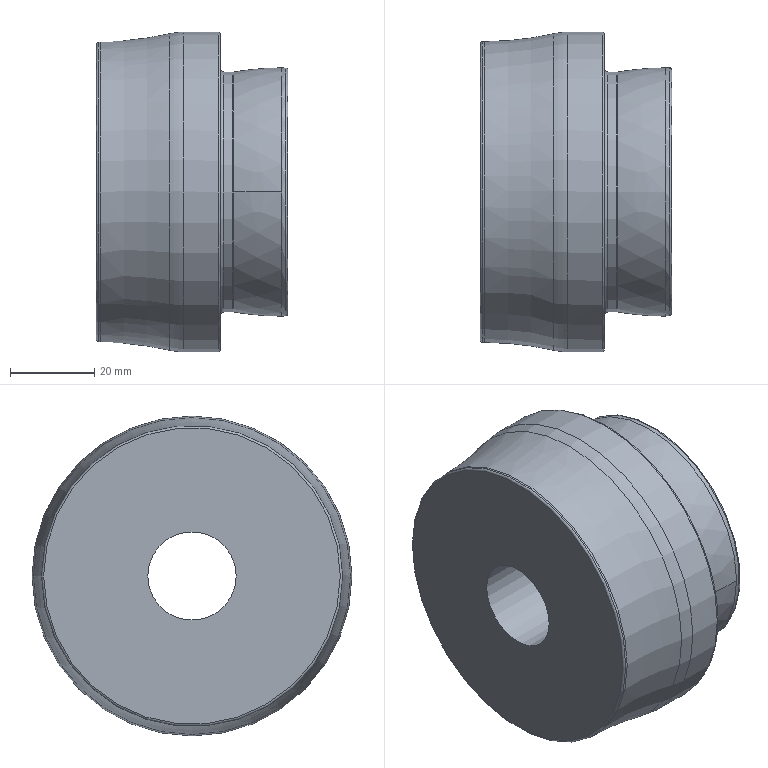Part | STEP file | P1317200001_D | 1 solid | 19 faces | box 45.5 x 76 x 76 mm | volume 152294 mm3 | torus 7 | cylinder 6 | plane 4 | spline 2 | commonest cylinder face diameters 21 x1 37 x1 57 x1 59 x1 71.5 x1 76 x1
STEP:
#1=CARTESIAN_POINT('',(0.,29.,0.));
#2=VERTEX_POINT('',#1);
#3=CARTESIAN_POINT('',(0.,28.999,-0.1765));
#4=VERTEX_POINT('',#3);
#5=CARTESIAN_POINT('',(0.,0.,0.));
#6=DIRECTION('',(1.,0.,0.));
#7=DIRECTION('',(0.,-1.,0.));
#8=AXIS2_PLACEMENT_3D('',#5,#6,#7);
#9=CIRCLE('',#8,29.);
#10=EDGE_CURVE('',#2,#4,#9,.T.);
#11=ORIENTED_EDGE('',*,*,#10,.T.);
#12=CARTESIAN_POINT('',(0.,0.,0.));
#13=DIRECTION('',(1.,0.,0.));
#14=DIRECTION('',(0.,-1.,0.));
#15=AXIS2_PLACEMENT_3D('',#12,#13,#14);
#16=CIRCLE('',#15,29.);
#17=EDGE_CURVE('',#4,#2,#16,.T.);
#18=ORIENTED_EDGE('',*,*,#17,.T.);
#19=EDGE_LOOP('',(#11,#18));
#20=FACE_OUTER_BOUND('',#19,.T.);
#21=CARTESIAN_POINT('',(0.,-18.5,0.));
#22=VERTEX_POINT('',#21);
#23=CARTESIAN_POINT('',(0.,0.,0.));
#24=DIRECTION('',(-1.,0.,0.));
#25=DIRECTION('',(0.,1.,0.));
#26=AXIS2_PLACEMENT_3D('',#23,#24,#25);
#27=CIRCLE('',#26,18.5);
#28=EDGE_CURVE('',#22,#22,#27,.T.);
#29=ORIENTED_EDGE('',*,*,#28,.T.);
#30=EDGE_LOOP('',(#29));
#31=FACE_BOUND('',#30,.T.);
#32=CARTESIAN_POINT('',(0.,0.,0.));
#33=DIRECTION('',(1.,0.,0.));
#34=DIRECTION('',(0.,-1.,0.));
#35=AXIS2_PLACEMENT_3D('',#32,#33,#34);
#36=PLANE('',#35);
#37=ADVANCED_FACE('',(#20,#31),#36,.T.);
#38=ORIENTED_EDGE('',*,*,#28,.F.);
#39=CARTESIAN_POINT('',(-2.,-18.5,0.));
#40=VERTEX_POINT('',#39);
#41=CARTESIAN_POINT('',(0.1,-18.5,0.));
#42=DIRECTION('',(-1.,0.,0.));
#43=VECTOR('',#42,18.5);
#44=LINE('',#41,#43);
#45=EDGE_CURVE('',#22,#40,#44,.T.);
#46=ORIENTED_EDGE('',*,*,#45,.T.);
#47=CARTESIAN_POINT('',(-2.,0.,0.));
#48=DIRECTION('',(-1.,0.,0.));
#49=DIRECTION('',(0.,1.,0.));
#50=AXIS2_PLACEMENT_3D('',#47,#48,#49);
#51=CIRCLE('',#50,18.5);
#52=EDGE_CURVE('',#40,#40,#51,.T.);
#53=ORIENTED_EDGE('',*,*,#52,.T.);
#54=ORIENTED_EDGE('',*,*,#45,.F.);
#55=EDGE_LOOP('',(#38,#46,#53,#54));
#56=FACE_OUTER_BOUND('',#55,.T.);
#57=CARTESIAN_POINT('',(0.1,0.,0.));
#58=DIRECTION('',(-1.,0.,0.));
#59=DIRECTION('',(0.,1.,0.));
#60=AXIS2_PLACEMENT_3D('',#57,#58,#59);
#61=CYLINDRICAL_SURFACE('',#60,18.5);
#62=ADVANCED_FACE('',(#56),#61,.F.);
#63=ORIENTED_EDGE('',*,*,#52,.F.);
#64=EDGE_LOOP('',(#63));
#65=FACE_OUTER_BOUND('',#64,.T.);
#66=CARTESIAN_POINT('',(-2.,-10.5,0.));
#67=VERTEX_POINT('',#66);
#68=CARTESIAN_POINT('',(-2.,10.5,0.));
#69=VERTEX_POINT('',#68);
#70=CARTESIAN_POINT('',(-2.,0.,0.));
#71=DIRECTION('',(-1.,0.,0.));
#72=DIRECTION('',(0.,1.,0.));
#73=AXIS2_PLACEMENT_3D('',#70,#71,#72);
#74=CIRCLE('',#73,10.5);
#75=EDGE_CURVE('',#67,#69,#74,.T.);
#76=ORIENTED_EDGE('',*,*,#75,.T.);
#77=CARTESIAN_POINT('',(-2.,0.,0.));
#78=DIRECTION('',(-1.,0.,0.));
#79=DIRECTION('',(0.,1.,0.));
#80=AXIS2_PLACEMENT_3D('',#77,#78,#79);
#81=CIRCLE('',#80,10.5);
#82=EDGE_CURVE('',#69,#67,#81,.T.);
#83=ORIENTED_EDGE('',*,*,#82,.T.);
#84=EDGE_LOOP('',(#76,#83));
#85=FACE_BOUND('',#84,.T.);
#86=CARTESIAN_POINT('',(-2.,0.,0.));
#87=DIRECTION('',(-1.,0.,0.));
#88=DIRECTION('',(0.,1.,0.));
#89=AXIS2_PLACEMENT_3D('',#86,#87,#88);
#90=PLANE('',#89);
#91=ADVANCED_FACE('',(#65,#85),#90,.F.);
#92=CARTESIAN_POINT('',(-45.5,-10.5,0.));
#93=VERTEX_POINT('',#92);
#94=CARTESIAN_POINT('',(-45.5,10.5,0.));
#95=VERTEX_POINT('',#94);
#96=CARTESIAN_POINT('',(-45.5,0.,0.));
#97=DIRECTION('',(-1.,0.,0.));
#98=DIRECTION('',(0.,1.,0.));
#99=AXIS2_PLACEMENT_3D('',#96,#97,#98);
#100=CIRCLE('',#99,10.5);
#101=EDGE_CURVE('',#93,#95,#100,.T.);
#102=ORIENTED_EDGE('',*,*,#101,.T.);
#103=CARTESIAN_POINT('',(-47.775,10.5,0.));
#104=DIRECTION('',(1.,0.,0.));
#105=VECTOR('',#104,10.5);
#106=LINE('',#103,#105);
#107=EDGE_CURVE('',#95,#69,#106,.T.);
#108=ORIENTED_EDGE('',*,*,#107,.T.);
#109=ORIENTED_EDGE('',*,*,#75,.F.);
#110=ORIENTED_EDGE('',*,*,#82,.F.);
#111=ORIENTED_EDGE('',*,*,#107,.F.);
#112=CARTESIAN_POINT('',(-45.5,0.,0.));
#113=DIRECTION('',(-1.,0.,0.));
#114=DIRECTION('',(0.,1.,0.));
#115=AXIS2_PLACEMENT_3D('',#112,#113,#114);
#116=CIRCLE('',#115,10.5);
#117=EDGE_CURVE('',#95,#93,#116,.T.);
#118=ORIENTED_EDGE('',*,*,#117,.T.);
#119=EDGE_LOOP('',(#102,#108,#109,#110,#111,#118));
#120=FACE_OUTER_BOUND('',#119,.T.);
#121=CARTESIAN_POINT('',(-47.775,0.,0.));
#122=DIRECTION('',(1.,0.,0.));
#123=DIRECTION('',(0.,-1.,0.));
#124=AXIS2_PLACEMENT_3D('',#121,#122,#123);
#125=CYLINDRICAL_SURFACE('',#124,10.5);
#126=ADVANCED_FACE('',(#120),#125,.F.);
#127=CARTESIAN_POINT('',(-45.5,35.25,0.));
#128=VERTEX_POINT('',#127);
#129=CARTESIAN_POINT('',(-45.5,35.249,0.2514));
#130=VERTEX_POINT('',#129);
#131=CARTESIAN_POINT('',(-45.5,0.,0.));
#132=DIRECTION('',(-1.,0.,0.));
#133=DIRECTION('',(0.,-1.,0.));
#134=AXIS2_PLACEMENT_3D('',#131,#132,#133);
#135=CIRCLE('',#134,35.25);
#136=EDGE_CURVE('',#128,#130,#135,.T.);
#137=ORIENTED_EDGE('',*,*,#136,.T.);
#138=CARTESIAN_POINT('',(-45.5,0.,0.));
#139=DIRECTION('',(-1.,0.,0.));
#140=DIRECTION('',(0.,-1.,0.));
#141=AXIS2_PLACEMENT_3D('',#138,#139,#140);
#142=CIRCLE('',#141,35.25);
#143=EDGE_CURVE('',#130,#128,#142,.T.);
#144=ORIENTED_EDGE('',*,*,#143,.T.);
#145=EDGE_LOOP('',(#137,#144));
#146=FACE_OUTER_BOUND('',#145,.T.);
#147=ORIENTED_EDGE('',*,*,#101,.F.);
#148=ORIENTED_EDGE('',*,*,#117,.F.);
#149=EDGE_LOOP('',(#147,#148));
#150=FACE_BOUND('',#149,.T.);
#151=CARTESIAN_POINT('',(-45.5,0.,0.));
#152=DIRECTION('',(1.,0.,0.));
#153=DIRECTION('',(0.,-1.,0.));
#154=AXIS2_PLACEMENT_3D('',#151,#152,#153);
#155=PLANE('',#154);
#156=ADVANCED_FACE('',(#146,#150),#155,.F.);
#157=CARTESIAN_POINT('',(-45.,35.75,0.));
#158=VERTEX_POINT('',#157);
#159=CARTESIAN_POINT('',(-45.,35.749,0.255));
#160=VERTEX_POINT('',#159);
#161=CARTESIAN_POINT('',(-45.,0.,0.));
#162=DIRECTION('',(-1.,0.,0.));
#163=DIRECTION('',(0.,-1.,0.));
#164=AXIS2_PLACEMENT_3D('',#161,#162,#163);
#165=CIRCLE('',#164,35.75);
#166=EDGE_CURVE('',#158,#160,#165,.T.);
#167=ORIENTED_EDGE('',*,*,#166,.T.);
#168=CARTESIAN_POINT('',(-45.,35.249,0.2514));
#169=DIRECTION('',(0.,-0.007133,1.));
#170=DIRECTION('',(0.,1.,0.007133));
#171=AXIS2_PLACEMENT_3D('',#168,#169,#170);
#172=CIRCLE('',#171,0.5);
#173=EDGE_CURVE('',#160,#130,#172,.T.);
#174=ORIENTED_EDGE('',*,*,#173,.T.);
#175=ORIENTED_EDGE('',*,*,#136,.F.);
#176=ORIENTED_EDGE('',*,*,#143,.F.);
#177=ORIENTED_EDGE('',*,*,#173,.F.);
#178=CARTESIAN_POINT('',(-45.,0.,0.));
#179=DIRECTION('',(-1.,0.,0.));
#180=DIRECTION('',(0.,-1.,0.));
#181=AXIS2_PLACEMENT_3D('',#178,#179,#180);
#182=CIRCLE('',#181,35.75);
#183=EDGE_CURVE('',#160,#158,#182,.T.);
#184=ORIENTED_EDGE('',*,*,#183,.T.);
#185=EDGE_LOOP('',(#167,#174,#175,#176,#177,#184));
#186=FACE_OUTER_BOUND('',#185,.T.);
#187=CARTESIAN_POINT('',(-45.,0.,0.));
#188=DIRECTION('',(1.,0.,0.));
#189=DIRECTION('',(0.,-1.,-0.007133));
#190=AXIS2_PLACEMENT_3D('',#187,#188,#189);
#191=TOROIDAL_SURFACE('',#190,35.25,0.5);
#192=ADVANCED_FACE('',(#186),#191,.T.);
#193=CARTESIAN_POINT('',(-44.5,-35.75,0.));
#194=VERTEX_POINT('',#193);
#195=CARTESIAN_POINT('',(-44.5,35.75,0.));
#196=VERTEX_POINT('',#195);
#197=CARTESIAN_POINT('',(-44.5,0.,0.));
#198=DIRECTION('',(-1.,0.,0.));
#199=DIRECTION('',(0.,1.,0.));
#200=AXIS2_PLACEMENT_3D('',#197,#198,#199);
#201=CIRCLE('',#200,35.75);
#202=EDGE_CURVE('',#194,#196,#201,.T.);
#203=ORIENTED_EDGE('',*,*,#202,.T.);
#204=CARTESIAN_POINT('',(-46.45,35.75,0.));
#205=DIRECTION('',(-1.,0.,0.));
#206=VECTOR('',#205,35.75);
#207=LINE('',#204,#206);
#208=EDGE_CURVE('',#196,#158,#207,.T.);
#209=ORIENTED_EDGE('',*,*,#208,.T.);
#210=ORIENTED_EDGE('',*,*,#183,.F.);
#211=ORIENTED_EDGE('',*,*,#166,.F.);
#212=ORIENTED_EDGE('',*,*,#208,.F.);
#213=CARTESIAN_POINT('',(-44.5,0.,0.));
#214=DIRECTION('',(-1.,0.,0.));
#215=DIRECTION('',(0.,1.,0.));
#216=AXIS2_PLACEMENT_3D('',#213,#214,#215);
#217=CIRCLE('',#216,35.75);
#218=EDGE_CURVE('',#196,#194,#217,.T.);
#219=ORIENTED_EDGE('',*,*,#218,.T.);
#220=EDGE_LOOP('',(#203,#209,#210,#211,#212,#219));
#221=FACE_OUTER_BOUND('',#220,.T.);
#222=CARTESIAN_POINT('',(-46.45,0.,0.));
#223=DIRECTION('',(1.,0.,0.));
#224=DIRECTION('',(0.,-1.,0.));
#225=AXIS2_PLACEMENT_3D('',#222,#223,#224);
#226=CYLINDRICAL_SURFACE('',#225,35.75);
#227=ADVANCED_FACE('',(#221),#226,.T.);
#228=CARTESIAN_POINT('',(-28.082,-37.617,0.));
#229=VERTEX_POINT('',#228);
#230=CARTESIAN_POINT('',(-28.082,37.617,0.));
#231=VERTEX_POINT('',#230);
#232=CARTESIAN_POINT('',(-28.082,0.,0.));
#233=DIRECTION('',(1.,0.,0.));
#234=DIRECTION('',(0.,1.,0.));
#235=AXIS2_PLACEMENT_3D('',#232,#233,#234);
#236=CIRCLE('',#235,37.617);
#237=EDGE_CURVE('',#229,#231,#236,.T.);
#238=ORIENTED_EDGE('',*,*,#237,.F.);
#239=CARTESIAN_POINT('',(-28.082,-37.617,0.186));
#240=VERTEX_POINT('',#239);
#241=CARTESIAN_POINT('',(-28.082,0.,0.));
#242=DIRECTION('',(1.,0.,0.));
#243=DIRECTION('',(0.,1.,0.));
#244=AXIS2_PLACEMENT_3D('',#241,#242,#243);
#245=CIRCLE('',#244,37.617);
#246=EDGE_CURVE('',#240,#229,#245,.T.);
#247=ORIENTED_EDGE('',*,*,#246,.F.);
#248=CARTESIAN_POINT('',(-28.082,0.,0.));
#249=DIRECTION('',(1.,0.,0.));
#250=DIRECTION('',(0.,1.,0.));
#251=AXIS2_PLACEMENT_3D('',#248,#249,#250);
#252=CIRCLE('',#251,37.617);
#253=EDGE_CURVE('',#231,#240,#252,.T.);
#254=ORIENTED_EDGE('',*,*,#253,.F.);
#255=CARTESIAN_POINT('',(-44.5,108.875,0.));
#256=DIRECTION('',(0.,0.,-1.));
#257=DIRECTION('',(0.,1.,0.));
#258=AXIS2_PLACEMENT_3D('',#255,#256,#257);
#259=CIRCLE('',#258,73.125);
#260=EDGE_CURVE('',#231,#196,#259,.T.);
#261=ORIENTED_EDGE('',*,*,#260,.T.);
#262=ORIENTED_EDGE('',*,*,#202,.F.);
#263=ORIENTED_EDGE('',*,*,#218,.F.);
#264=ORIENTED_EDGE('',*,*,#260,.F.);
#265=EDGE_LOOP('',(#238,#247,#254,#261,#262,#263,#264));
#266=FACE_OUTER_BOUND('',#265,.T.);
#267=CARTESIAN_POINT('',(-44.5,0.,0.));
#268=DIRECTION('',(1.,0.,0.));
#269=DIRECTION('',(0.,-1.,0.));
#270=AXIS2_PLACEMENT_3D('',#267,#268,#269);
#271=TOROIDAL_SURFACE('',#270,108.875,73.125);
#272=ADVANCED_FACE('',(#266),#271,.F.);
#273=CARTESIAN_POINT('',(-24.714,-38.,0.));
#274=VERTEX_POINT('',#273);
#275=CARTESIAN_POINT('',(-24.714,38.,0.));
#276=VERTEX_POINT('',#275);
#277=CARTESIAN_POINT('',(-24.714,0.,0.));
#278=DIRECTION('',(1.,0.,0.));
#279=DIRECTION('',(0.,1.,0.));
#280=AXIS2_PLACEMENT_3D('',#277,#278,#279);
#281=CIRCLE('',#280,38.);
#282=EDGE_CURVE('',#274,#276,#281,.T.);
#283=ORIENTED_EDGE('',*,*,#282,.F.);
#284=CARTESIAN_POINT('',(-24.714,-38.,0.1878));
#285=VERTEX_POINT('',#284);
#286=CARTESIAN_POINT('',(-24.714,0.,0.));
#287=DIRECTION('',(1.,0.,0.));
#288=DIRECTION('',(0.,1.,0.));
#289=AXIS2_PLACEMENT_3D('',#286,#287,#288);
#290=CIRCLE('',#289,38.);
#291=EDGE_CURVE('',#285,#274,#290,.T.);
#292=ORIENTED_EDGE('',*,*,#291,.F.);
#293=CARTESIAN_POINT('',(-24.714,-23.,0.1137));
#294=DIRECTION('',(0.,-0.004943,-1.));
#295=DIRECTION('',(0.,-1.,0.004943));
#296=AXIS2_PLACEMENT_3D('',#293,#294,#295);
#297=CIRCLE('',#296,15.);
#298=EDGE_CURVE('',#285,#240,#297,.T.);
#299=ORIENTED_EDGE('',*,*,#298,.T.);
#300=ORIENTED_EDGE('',*,*,#246,.T.);
#301=ORIENTED_EDGE('',*,*,#237,.T.);
#302=ORIENTED_EDGE('',*,*,#253,.T.);
#303=ORIENTED_EDGE('',*,*,#298,.F.);
#304=CARTESIAN_POINT('',(-24.714,0.,0.));
#305=DIRECTION('',(1.,0.,0.));
#306=DIRECTION('',(0.,1.,0.));
#307=AXIS2_PLACEMENT_3D('',#304,#305,#306);
#308=CIRCLE('',#307,38.);
#309=EDGE_CURVE('',#276,#285,#308,.T.);
#310=ORIENTED_EDGE('',*,*,#309,.F.);
#311=EDGE_LOOP('',(#283,#292,#299,#300,#301,#302,#303,#310));
#312=FACE_OUTER_BOUND('',#311,.T.);
#313=CARTESIAN_POINT('',(-24.714,0.,0.));
#314=DIRECTION('',(1.,0.,0.));
#315=DIRECTION('',(0.,1.,-0.004943));
#316=AXIS2_PLACEMENT_3D('',#313,#314,#315);
#317=TOROIDAL_SURFACE('',#316,23.,15.);
#318=ADVANCED_FACE('',(#312),#317,.T.);
#319=CARTESIAN_POINT('',(-16.5,-38.,0.));
#320=VERTEX_POINT('',#319);
#321=CARTESIAN_POINT('',(-16.5,38.,0.1726));
#322=VERTEX_POINT('',#321);
#323=CARTESIAN_POINT('',(-16.5,0.,0.));
#324=DIRECTION('',(-1.,0.,0.));
#325=DIRECTION('',(0.,-1.,0.));
#326=AXIS2_PLACEMENT_3D('',#323,#324,#325);
#327=CIRCLE('',#326,38.);
#328=EDGE_CURVE('',#320,#322,#327,.T.);
#329=ORIENTED_EDGE('',*,*,#328,.T.);
#330=CARTESIAN_POINT('',(-16.5,38.,0.));
#331=VERTEX_POINT('',#330);
#332=CARTESIAN_POINT('',(-16.5,0.,0.));
#333=DIRECTION('',(-1.,0.,0.));
#334=DIRECTION('',(0.,-1.,0.));
#335=AXIS2_PLACEMENT_3D('',#332,#333,#334);
#336=CIRCLE('',#335,38.);
#337=EDGE_CURVE('',#322,#331,#336,.T.);
#338=ORIENTED_EDGE('',*,*,#337,.T.);
#339=CARTESIAN_POINT('',(-47.775,38.,0.));
#340=DIRECTION('',(-1.,0.,0.));
#341=VECTOR('',#340,38.);
#342=LINE('',#339,#341);
#343=EDGE_CURVE('',#331,#276,#342,.T.);
#344=ORIENTED_EDGE('',*,*,#343,.T.);
#345=ORIENTED_EDGE('',*,*,#309,.T.);
#346=ORIENTED_EDGE('',*,*,#291,.T.);
#347=ORIENTED_EDGE('',*,*,#282,.T.);
#348=ORIENTED_EDGE('',*,*,#343,.F.);
#349=CARTESIAN_POINT('',(-16.5,0.,0.));
#350=DIRECTION('',(-1.,0.,0.));
#351=DIRECTION('',(0.,-1.,0.));
#352=AXIS2_PLACEMENT_3D('',#349,#350,#351);
#353=CIRCLE('',#352,38.);
#354=EDGE_CURVE('',#331,#320,#353,.T.);
#355=ORIENTED_EDGE('',*,*,#354,.T.);
#356=EDGE_LOOP('',(#329,#338,#344,#345,#346,#347,#348,#355));
#357=FACE_OUTER_BOUND('',#356,.T.);
#358=CARTESIAN_POINT('',(-47.775,0.,0.));
#359=DIRECTION('',(1.,0.,0.));
#360=DIRECTION('',(0.,-1.,0.));
#361=AXIS2_PLACEMENT_3D('',#358,#359,#360);
#362=CYLINDRICAL_SURFACE('',#361,38.);
#363=ADVANCED_FACE('',(#357),#362,.T.);
#364=CARTESIAN_POINT('',(-16.,37.5,0.));
#365=VERTEX_POINT('',#364);
#366=CARTESIAN_POINT('',(-16.,37.5,0.1703));
#367=VERTEX_POINT('',#366);
#368=CARTESIAN_POINT('',(-16.,0.,0.));
#369=DIRECTION('',(-1.,0.,0.));
#370=DIRECTION('',(0.,-1.,0.));
#371=AXIS2_PLACEMENT_3D('',#368,#369,#370);
#372=CIRCLE('',#371,37.5);
#373=EDGE_CURVE('',#365,#367,#372,.T.);
#374=ORIENTED_EDGE('',*,*,#373,.T.);
#375=CARTESIAN_POINT('',(-16.5,37.5,0.1703));
#376=DIRECTION('',(0.,-0.004542,1.));
#377=DIRECTION('',(0.,1.,0.004542));
#378=AXIS2_PLACEMENT_3D('',#375,#376,#377);
#379=CIRCLE('',#378,0.5);
#380=EDGE_CURVE('',#367,#322,#379,.T.);
#381=ORIENTED_EDGE('',*,*,#380,.T.);
#382=ORIENTED_EDGE('',*,*,#328,.F.);
#383=ORIENTED_EDGE('',*,*,#354,.F.);
#384=ORIENTED_EDGE('',*,*,#337,.F.);
#385=ORIENTED_EDGE('',*,*,#380,.F.);
#386=CARTESIAN_POINT('',(-16.,0.,0.));
#387=DIRECTION('',(-1.,0.,0.));
#388=DIRECTION('',(0.,-1.,0.));
#389=AXIS2_PLACEMENT_3D('',#386,#387,#388);
#390=CIRCLE('',#389,37.5);
#391=EDGE_CURVE('',#367,#365,#390,.T.);
#392=ORIENTED_EDGE('',*,*,#391,.T.);
#393=EDGE_LOOP('',(#374,#381,#382,#383,#384,#385,#392));
#394=FACE_OUTER_BOUND('',#393,.T.);
#395=CARTESIAN_POINT('',(-16.5,0.,0.));
#396=DIRECTION('',(1.,0.,0.));
#397=DIRECTION('',(0.,-1.,-0.004542));
#398=AXIS2_PLACEMENT_3D('',#395,#396,#397);
#399=TOROIDAL_SURFACE('',#398,37.5,0.5);
#400=ADVANCED_FACE('',(#394),#399,.T.);
#401=ORIENTED_EDGE('',*,*,#373,.F.);
#402=ORIENTED_EDGE('',*,*,#391,.F.);
#403=EDGE_LOOP('',(#401,#402));
#404=FACE_OUTER_BOUND('',#403,.T.);
#405=CARTESIAN_POINT('',(-16.,-29.3,0.));
#406=VERTEX_POINT('',#405);
#407=CARTESIAN_POINT('',(-16.,29.299,0.1775));
#408=VERTEX_POINT('',#407);
#409=CARTESIAN_POINT('',(-16.,0.,0.));
#410=DIRECTION('',(-1.,0.,0.));
#411=DIRECTION('',(0.,-1.,0.));
#412=AXIS2_PLACEMENT_3D('',#409,#410,#411);
#413=CIRCLE('',#412,29.3);
#414=EDGE_CURVE('',#406,#408,#413,.T.);
#415=ORIENTED_EDGE('',*,*,#414,.T.);
#416=CARTESIAN_POINT('',(-16.,0.,0.));
#417=DIRECTION('',(-1.,0.,0.));
#418=DIRECTION('',(0.,-1.,0.));
#419=AXIS2_PLACEMENT_3D('',#416,#417,#418);
#420=CIRCLE('',#419,29.3);
#421=EDGE_CURVE('',#408,#406,#420,.T.);
#422=ORIENTED_EDGE('',*,*,#421,.T.);
#423=EDGE_LOOP('',(#415,#422));
#424=FACE_BOUND('',#423,.T.);
#425=CARTESIAN_POINT('',(-16.,0.,0.));
#426=DIRECTION('',(1.,0.,0.));
#427=DIRECTION('',(0.,-1.,0.));
#428=AXIS2_PLACEMENT_3D('',#425,#426,#427);
#429=PLANE('',#428);
#430=ADVANCED_FACE('',(#404,#424),#429,.T.);
#431=CARTESIAN_POINT('',(-15.2,-28.5,0.));
#432=VERTEX_POINT('',#431);
#433=CARTESIAN_POINT('',(-15.2,28.499,0.1726));
#434=VERTEX_POINT('',#433);
#435=CARTESIAN_POINT('',(-15.2,0.,0.));
#436=DIRECTION('',(-1.,0.,0.));
#437=DIRECTION('',(0.,-1.,0.));
#438=AXIS2_PLACEMENT_3D('',#435,#436,#437);
#439=CIRCLE('',#438,28.5);
#440=EDGE_CURVE('',#432,#434,#439,.T.);
#441=ORIENTED_EDGE('',*,*,#440,.T.);
#442=CARTESIAN_POINT('',(-15.2,29.299,0.1775));
#443=DIRECTION('',(0.,0.006056,-1.));
#444=DIRECTION('',(0.,1.,0.006056));
#445=AXIS2_PLACEMENT_3D('',#442,#443,#444);
#446=CIRCLE('',#445,0.8);
#447=EDGE_CURVE('',#434,#408,#446,.T.);
#448=ORIENTED_EDGE('',*,*,#447,.T.);
#449=ORIENTED_EDGE('',*,*,#414,.F.);
#450=ORIENTED_EDGE('',*,*,#421,.F.);
#451=ORIENTED_EDGE('',*,*,#447,.F.);
#452=CARTESIAN_POINT('',(-15.2,28.5,0.));
#453=VERTEX_POINT('',#452);
#454=CARTESIAN_POINT('',(-15.2,0.,0.));
#455=DIRECTION('',(-1.,0.,0.));
#456=DIRECTION('',(0.,-1.,0.));
#457=AXIS2_PLACEMENT_3D('',#454,#455,#456);
#458=CIRCLE('',#457,28.5);
#459=EDGE_CURVE('',#434,#453,#458,.T.);
#460=ORIENTED_EDGE('',*,*,#459,.T.);
#461=CARTESIAN_POINT('',(-15.2,0.,0.));
#462=DIRECTION('',(-1.,0.,0.));
#463=DIRECTION('',(0.,-1.,0.));
#464=AXIS2_PLACEMENT_3D('',#461,#462,#463);
#465=CIRCLE('',#464,28.5);
#466=EDGE_CURVE('',#453,#432,#465,.T.);
#467=ORIENTED_EDGE('',*,*,#466,.T.);
#468=EDGE_LOOP('',(#441,#448,#449,#450,#451,#460,#467));
#469=FACE_OUTER_BOUND('',#468,.T.);
#470=CARTESIAN_POINT('',(-15.2,0.,0.));
#471=DIRECTION('',(1.,0.,0.));
#472=DIRECTION('',(0.,-1.,-0.006056));
#473=AXIS2_PLACEMENT_3D('',#470,#471,#472);
#474=TOROIDAL_SURFACE('',#473,29.3,0.8);
#475=ADVANCED_FACE('',(#469),#474,.F.);
#476=CARTESIAN_POINT('',(-13.052,-28.5,0.));
#477=VERTEX_POINT('',#476);
#478=CARTESIAN_POINT('',(-13.052,28.5,0.1682));
#479=VERTEX_POINT('',#478);
#480=CARTESIAN_POINT('',(-13.052,0.,0.));
#481=DIRECTION('',(-1.,0.,0.));
#482=DIRECTION('',(0.,-1.,0.));
#483=AXIS2_PLACEMENT_3D('',#480,#481,#482);
#484=CIRCLE('',#483,28.5);
#485=EDGE_CURVE('',#477,#479,#484,.T.);
#486=ORIENTED_EDGE('',*,*,#485,.T.);
#487=CARTESIAN_POINT('',(-13.052,28.5,0.));
#488=VERTEX_POINT('',#487);
#489=CARTESIAN_POINT('',(-13.052,0.,0.));
#490=DIRECTION('',(-1.,0.,0.));
#491=DIRECTION('',(0.,-1.,0.));
#492=AXIS2_PLACEMENT_3D('',#489,#490,#491);
#493=CIRCLE('',#492,28.5);
#494=EDGE_CURVE('',#479,#488,#493,.T.);
#495=ORIENTED_EDGE('',*,*,#494,.T.);
#496=CARTESIAN_POINT('',(-16.8,28.5,0.));
#497=DIRECTION('',(-1.,0.,0.));
#498=VECTOR('',#497,28.5);
#499=LINE('',#496,#498);
#500=EDGE_CURVE('',#488,#453,#499,.T.);
#501=ORIENTED_EDGE('',*,*,#500,.T.);
#502=ORIENTED_EDGE('',*,*,#459,.F.);
#503=ORIENTED_EDGE('',*,*,#440,.F.);
#504=ORIENTED_EDGE('',*,*,#466,.F.);
#505=ORIENTED_EDGE('',*,*,#500,.F.);
#506=CARTESIAN_POINT('',(-13.052,0.,0.));
#507=DIRECTION('',(-1.,0.,0.));
#508=DIRECTION('',(0.,-1.,0.));
#509=AXIS2_PLACEMENT_3D('',#506,#507,#508);
#510=CIRCLE('',#509,28.5);
#511=EDGE_CURVE('',#488,#477,#510,.T.);
#512=ORIENTED_EDGE('',*,*,#511,.T.);
#513=EDGE_LOOP('',(#486,#495,#501,#502,#503,#504,#505,#512));
#514=FACE_OUTER_BOUND('',#513,.T.);
#515=CARTESIAN_POINT('',(-16.8,0.,0.));
#516=DIRECTION('',(1.,0.,0.));
#517=DIRECTION('',(0.,-1.,0.));
#518=AXIS2_PLACEMENT_3D('',#515,#516,#517);
#519=CYLINDRICAL_SURFACE('',#518,28.5);
#520=ADVANCED_FACE('',(#514),#519,.T.);
#521=CARTESIAN_POINT('',(-12.949,-28.509,0.));
#522=VERTEX_POINT('',#521);
#523=CARTESIAN_POINT('',(-12.949,28.508,0.1682));
#524=VERTEX_POINT('',#523);
#525=CARTESIAN_POINT('',(-12.949,0.,0.));
#526=DIRECTION('',(-1.,0.,0.));
#527=DIRECTION('',(0.,-1.,0.));
#528=AXIS2_PLACEMENT_3D('',#525,#526,#527);
#529=CIRCLE('',#528,28.509);
#530=EDGE_CURVE('',#522,#524,#529,.T.);
#531=ORIENTED_EDGE('',*,*,#530,.T.);
#532=CARTESIAN_POINT('',(-13.052,29.099,0.1717));
#533=DIRECTION('',(0.,0.005901,-1.));
#534=DIRECTION('',(0.,1.,0.005901));
#535=AXIS2_PLACEMENT_3D('',#532,#533,#534);
#536=CIRCLE('',#535,0.6);
#537=EDGE_CURVE('',#524,#479,#536,.T.);
#538=ORIENTED_EDGE('',*,*,#537,.T.);
#539=ORIENTED_EDGE('',*,*,#485,.F.);
#540=ORIENTED_EDGE('',*,*,#511,.F.);
#541=ORIENTED_EDGE('',*,*,#494,.F.);
#542=ORIENTED_EDGE('',*,*,#537,.F.);
#543=CARTESIAN_POINT('',(-12.949,28.509,0.));
#544=VERTEX_POINT('',#543);
#545=CARTESIAN_POINT('',(-12.949,0.,0.));
#546=DIRECTION('',(-1.,0.,0.));
#547=DIRECTION('',(0.,-1.,0.));
#548=AXIS2_PLACEMENT_3D('',#545,#546,#547);
#549=CIRCLE('',#548,28.509);
#550=EDGE_CURVE('',#524,#544,#549,.T.);
#551=ORIENTED_EDGE('',*,*,#550,.T.);
#552=CARTESIAN_POINT('',(-12.949,0.,0.));
#553=DIRECTION('',(-1.,0.,0.));
#554=DIRECTION('',(0.,1.,0.));
#555=AXIS2_PLACEMENT_3D('',#552,#553,#554);
#556=CIRCLE('',#555,28.509);
#557=EDGE_CURVE('',#544,#522,#556,.T.);
#558=ORIENTED_EDGE('',*,*,#557,.T.);
#559=EDGE_LOOP('',(#531,#538,#539,#540,#541,#542,#551,#558));
#560=FACE_OUTER_BOUND('',#559,.T.);
#561=CARTESIAN_POINT('',(-13.052,0.,0.));
#562=DIRECTION('',(1.,0.,0.));
#563=DIRECTION('',(0.,-1.,-0.005901));
#564=AXIS2_PLACEMENT_3D('',#561,#562,#563);
#565=TOROIDAL_SURFACE('',#564,29.1,0.6);
#566=ADVANCED_FACE('',(#560),#565,.F.);
#567=ORIENTED_EDGE('',*,*,#530,.F.);
#568=CARTESIAN_POINT('',(-1.5,-29.5,0.));
#569=VERTEX_POINT('',#568);
#570=CARTESIAN_POINT('',(-1.5,37.125,0.));
#571=DIRECTION('',(0.,0.,1.));
#572=DIRECTION('',(-0.1718,-0.9851,0.));
#573=AXIS2_PLACEMENT_3D('',#570,#571,#572);
#574=CIRCLE('',#573,66.625);
#575=EDGE_CURVE('',#522,#569,#574,.T.);
#576=ORIENTED_EDGE('',*,*,#575,.T.);
#577=CARTESIAN_POINT('',(-1.5,29.5,0.));
#578=VERTEX_POINT('',#577);
#579=CARTESIAN_POINT('',(-1.5,0.,0.));
#580=DIRECTION('',(1.,0.,0.));
#581=DIRECTION('',(0.,1.,0.));
#582=AXIS2_PLACEMENT_3D('',#579,#580,#581);
#583=CIRCLE('',#582,29.5);
#584=EDGE_CURVE('',#578,#569,#583,.T.);
#585=ORIENTED_EDGE('',*,*,#584,.F.);
#586=CARTESIAN_POINT('',(-1.5,-37.125,0.));
#587=DIRECTION('',(0.,0.,-1.));
#588=DIRECTION('',(-0.1718,0.9851,0.));
#589=AXIS2_PLACEMENT_3D('',#586,#587,#588);
#590=CIRCLE('',#589,66.625);
#591=EDGE_CURVE('',#544,#578,#590,.T.);
#592=ORIENTED_EDGE('',*,*,#591,.F.);
#593=ORIENTED_EDGE('',*,*,#550,.F.);
#594=EDGE_LOOP('',(#567,#576,#585,#592,#593));
#595=FACE_OUTER_BOUND('',#594,.T.);
#596=CARTESIAN_POINT('',(-13.176,28.413,-1.788));
#597=CARTESIAN_POINT('',(-9.243,29.111,-1.832));
#598=CARTESIAN_POINT('',(-5.264,29.455,-1.853));
#599=CARTESIAN_POINT('',(-1.27,29.441,-1.852));
#600=CARTESIAN_POINT('',(-13.176,29.513,15.698));
#601=CARTESIAN_POINT('',(-9.243,30.238,16.084));
#602=CARTESIAN_POINT('',(-5.264,30.596,16.274));
#603=CARTESIAN_POINT('',(-1.27,30.581,16.266));
#604=CARTESIAN_POINT('',(-13.176,17.52,28.469));
#605=CARTESIAN_POINT('',(-9.243,17.951,29.169));
#606=CARTESIAN_POINT('',(-5.264,18.163,29.513));
#607=CARTESIAN_POINT('',(-1.27,18.154,29.5));
#608=CARTESIAN_POINT('',(-13.176,0.,28.469));
#609=CARTESIAN_POINT('',(-9.243,0.,29.169));
#610=CARTESIAN_POINT('',(-5.264,0.,29.513));
#611=CARTESIAN_POINT('',(-1.27,0.,29.5));
#612=CARTESIAN_POINT('',(-13.176,-17.52,28.469));
#613=CARTESIAN_POINT('',(-9.243,-17.951,29.169));
#614=CARTESIAN_POINT('',(-5.264,-18.163,29.513));
#615=CARTESIAN_POINT('',(-1.27,-18.154,29.5));
#616=CARTESIAN_POINT('',(-13.176,-29.513,15.698));
#617=CARTESIAN_POINT('',(-9.243,-30.238,16.084));
#618=CARTESIAN_POINT('',(-5.264,-30.596,16.274));
#619=CARTESIAN_POINT('',(-1.27,-30.581,16.266));
#620=CARTESIAN_POINT('',(-13.176,-28.413,-1.788));
#621=CARTESIAN_POINT('',(-9.243,-29.111,-1.832));
#622=CARTESIAN_POINT('',(-5.264,-29.455,-1.853));
#623=CARTESIAN_POINT('',(-1.27,-29.441,-1.852));
#624=(BOUNDED_SURFACE()B_SPLINE_SURFACE(3,3,((#596,#597,#598,#599),(#600,#601,#602,#603),(#604,#605,#606,#607),(#608,#609,#610,#611),(#612,#613,#614,#615),(#616,#617,#618,#619),(#620,#621,#622,#623)),.UNSPECIFIED.,.F.,.F.,.F.)B_SPLINE_SURFACE_WITH_KNOTS((4,3,4),(4,4),(0.,1.,2.),(0.,1.),.UNSPECIFIED.)GEOMETRIC_REPRESENTATION_ITEM()RATIONAL_B_SPLINE_SURFACE(((1.19,1.186,1.186,1.19),(0.9395,0.9369,0.9369,0.9395),(0.9395,0.9369,0.9369,0.9395),(1.19,1.186,1.186,1.19),(0.9395,0.9369,0.9369,0.9395),(0.9395,0.9369,0.9369,0.9395),(1.19,1.186,1.186,1.19)))REPRESENTATION_ITEM('')SURFACE());
#625=ADVANCED_FACE('',(#595),#624,.T.);
#626=ORIENTED_EDGE('',*,*,#557,.F.);
#627=ORIENTED_EDGE('',*,*,#591,.T.);
#628=CARTESIAN_POINT('',(-1.5,0.,0.));
#629=DIRECTION('',(1.,0.,0.));
#630=DIRECTION('',(0.,-1.,0.));
#631=AXIS2_PLACEMENT_3D('',#628,#629,#630);
#632=CIRCLE('',#631,29.5);
#633=EDGE_CURVE('',#569,#578,#632,.T.);
#634=ORIENTED_EDGE('',*,*,#633,.F.);
#635=ORIENTED_EDGE('',*,*,#575,.F.);
#636=EDGE_LOOP('',(#626,#627,#634,#635));
#637=FACE_OUTER_BOUND('',#636,.T.);
#638=CARTESIAN_POINT('',(-13.176,-28.413,1.788));
#639=CARTESIAN_POINT('',(-9.243,-29.111,1.832));
#640=CARTESIAN_POINT('',(-5.264,-29.455,1.853));
#641=CARTESIAN_POINT('',(-1.27,-29.441,1.852));
#642=CARTESIAN_POINT('',(-13.176,-29.513,-15.698));
#643=CARTESIAN_POINT('',(-9.243,-30.238,-16.084));
#644=CARTESIAN_POINT('',(-5.264,-30.596,-16.274));
#645=CARTESIAN_POINT('',(-1.27,-30.581,-16.266));
#646=CARTESIAN_POINT('',(-13.176,-17.52,-28.469));
#647=CARTESIAN_POINT('',(-9.243,-17.951,-29.169));
#648=CARTESIAN_POINT('',(-5.264,-18.163,-29.513));
#649=CARTESIAN_POINT('',(-1.27,-18.154,-29.5));
#650=CARTESIAN_POINT('',(-13.176,0.,-28.469));
#651=CARTESIAN_POINT('',(-9.243,0.,-29.169));
#652=CARTESIAN_POINT('',(-5.264,0.,-29.513));
#653=CARTESIAN_POINT('',(-1.27,0.,-29.5));
#654=CARTESIAN_POINT('',(-13.176,17.52,-28.469));
#655=CARTESIAN_POINT('',(-9.243,17.951,-29.169));
#656=CARTESIAN_POINT('',(-5.264,18.163,-29.513));
#657=CARTESIAN_POINT('',(-1.27,18.154,-29.5));
#658=CARTESIAN_POINT('',(-13.176,29.513,-15.698));
#659=CARTESIAN_POINT('',(-9.243,30.238,-16.084));
#660=CARTESIAN_POINT('',(-5.264,30.596,-16.274));
#661=CARTESIAN_POINT('',(-1.27,30.581,-16.266));
#662=CARTESIAN_POINT('',(-13.176,28.413,1.788));
#663=CARTESIAN_POINT('',(-9.243,29.111,1.832));
#664=CARTESIAN_POINT('',(-5.264,29.455,1.853));
#665=CARTESIAN_POINT('',(-1.27,29.441,1.852));
#666=(BOUNDED_SURFACE()B_SPLINE_SURFACE(3,3,((#638,#639,#640,#641),(#642,#643,#644,#645),(#646,#647,#648,#649),(#650,#651,#652,#653),(#654,#655,#656,#657),(#658,#659,#660,#661),(#662,#663,#664,#665)),.UNSPECIFIED.,.F.,.F.,.F.)B_SPLINE_SURFACE_WITH_KNOTS((4,3,4),(4,4),(0.,1.,2.),(0.,1.),.UNSPECIFIED.)GEOMETRIC_REPRESENTATION_ITEM()RATIONAL_B_SPLINE_SURFACE(((1.19,1.186,1.186,1.19),(0.9395,0.9369,0.9369,0.9395),(0.9395,0.9369,0.9369,0.9395),(1.19,1.186,1.186,1.19),(0.9395,0.9369,0.9369,0.9395),(0.9395,0.9369,0.9369,0.9395),(1.19,1.186,1.186,1.19)))REPRESENTATION_ITEM('')SURFACE());
#667=ADVANCED_FACE('',(#637),#666,.T.);
#668=CARTESIAN_POINT('',(-0.5,29.5,0.));
#669=VERTEX_POINT('',#668);
#670=CARTESIAN_POINT('',(-0.5,29.499,-0.1795));
#671=VERTEX_POINT('',#670);
#672=CARTESIAN_POINT('',(-0.5,0.,0.));
#673=DIRECTION('',(1.,0.,0.));
#674=DIRECTION('',(0.,-1.,0.));
#675=AXIS2_PLACEMENT_3D('',#672,#673,#674);
#676=CIRCLE('',#675,29.5);
#677=EDGE_CURVE('',#669,#671,#676,.T.);
#678=ORIENTED_EDGE('',*,*,#677,.F.);
#679=CARTESIAN_POINT('',(-16.8,29.5,0.));
#680=DIRECTION('',(-1.,0.,0.));
#681=VECTOR('',#680,29.5);
#682=LINE('',#679,#681);
#683=EDGE_CURVE('',#669,#578,#682,.T.);
#684=ORIENTED_EDGE('',*,*,#683,.T.);
#685=ORIENTED_EDGE('',*,*,#584,.T.);
#686=ORIENTED_EDGE('',*,*,#633,.T.);
#687=ORIENTED_EDGE('',*,*,#683,.F.);
#688=CARTESIAN_POINT('',(-0.5,0.,0.));
#689=DIRECTION('',(1.,0.,0.));
#690=DIRECTION('',(0.,-1.,0.));
#691=AXIS2_PLACEMENT_3D('',#688,#689,#690);
#692=CIRCLE('',#691,29.5);
#693=EDGE_CURVE('',#671,#669,#692,.T.);
#694=ORIENTED_EDGE('',*,*,#693,.F.);
#695=EDGE_LOOP('',(#678,#684,#685,#686,#687,#694));
#696=FACE_OUTER_BOUND('',#695,.T.);
#697=CARTESIAN_POINT('',(-16.8,0.,0.));
#698=DIRECTION('',(1.,0.,0.));
#699=DIRECTION('',(0.,-1.,0.));
#700=AXIS2_PLACEMENT_3D('',#697,#698,#699);
#701=CYLINDRICAL_SURFACE('',#700,29.5);
#702=ADVANCED_FACE('',(#696),#701,.T.);
#703=ORIENTED_EDGE('',*,*,#10,.F.);
#704=ORIENTED_EDGE('',*,*,#17,.F.);
#705=CARTESIAN_POINT('',(-0.5,28.999,-0.1765));
#706=DIRECTION('',(0.,0.006085,1.));
#707=DIRECTION('',(0.,1.,-0.006085));
#708=AXIS2_PLACEMENT_3D('',#705,#706,#707);
#709=CIRCLE('',#708,0.5);
#710=EDGE_CURVE('',#4,#671,#709,.T.);
#711=ORIENTED_EDGE('',*,*,#710,.T.);
#712=ORIENTED_EDGE('',*,*,#693,.T.);
#713=ORIENTED_EDGE('',*,*,#677,.T.);
#714=ORIENTED_EDGE('',*,*,#710,.F.);
#715=EDGE_LOOP('',(#703,#704,#711,#712,#713,#714));
#716=FACE_OUTER_BOUND('',#715,.T.);
#717=CARTESIAN_POINT('',(-0.5,0.,0.));
#718=DIRECTION('',(1.,0.,0.));
#719=DIRECTION('',(0.,-1.,0.006085));
#720=AXIS2_PLACEMENT_3D('',#717,#718,#719);
#721=TOROIDAL_SURFACE('',#720,29.,0.5);
#722=ADVANCED_FACE('',(#716),#721,.T.);
#723=CLOSED_SHELL('',(#37,#62,#91,#126,#156,#192,#227,#272,#318,#363,#400,#430,#475,#520,#566,#625,#667,#702,#722));
#724=MANIFOLD_SOLID_BREP('',#723);
#725=(LENGTH_UNIT()NAMED_UNIT(*)SI_UNIT(.MILLI.,.METRE.));
#726=UNCERTAINTY_MEASURE_WITH_UNIT(LENGTH_MEASURE(0.01),#725,'','');
#727=(NAMED_UNIT(*)PLANE_ANGLE_UNIT()SI_UNIT($,.RADIAN.));
#728=(NAMED_UNIT(*)SI_UNIT($,.STERADIAN.)SOLID_ANGLE_UNIT());
#729=(GEOMETRIC_REPRESENTATION_CONTEXT(3)GLOBAL_UNCERTAINTY_ASSIGNED_CONTEXT((#726))GLOBAL_UNIT_ASSIGNED_CONTEXT((#725,#727,#728))REPRESENTATION_CONTEXT('',''));
#730=ADVANCED_BREP_SHAPE_REPRESENTATION('',(#724),#729);